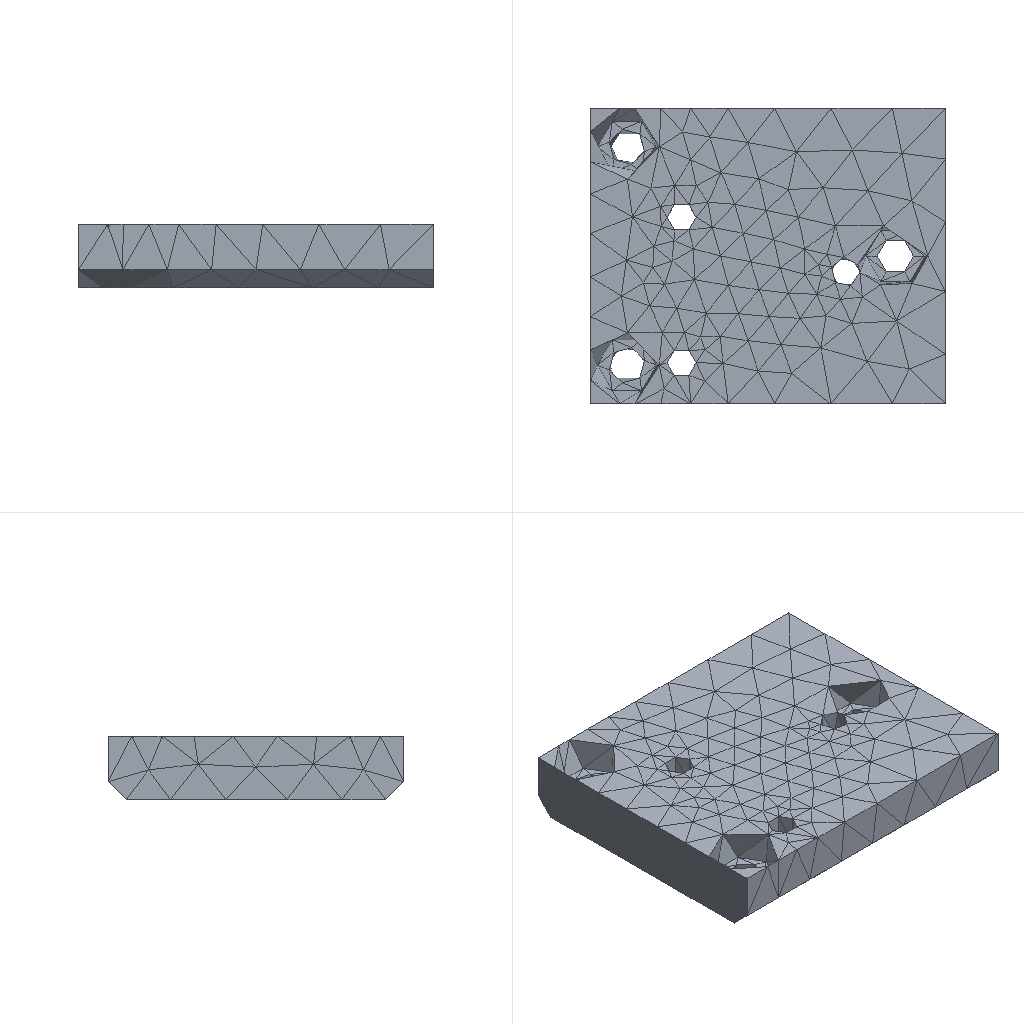Simulation study | nx simcenter
Set-up summary:
category,name,step,type,value,unit,region
solver,nx_nastran (Simcenter)
units,not stated in the deck,,not stated
analysis,deck,,static,static
analysis,solution,,SOL,101
load_step,SUBCASE 1,1,SUBCASE,SPC=1 LOAD=2
load_step,requested,,,1
mesh,nodes,,,2321
mesh,elements,,,1159
element_type,CTETRA,,solid,1159
load,nodal force total,,FX,0.0,model units
load,nodal force total,,FY,0.0,model units
load,nodal force total,,FZ,5000000.063,model units
load,load commands in deck,,count,388
bc,support commands in deck,,count,462
analysis,NX solution 0,,Structural,Linear Statics - Single Constraint
check,setup vs results,,match,every grid point's frame and coordinates and every element id; grid points of CTETRA elements
Nastran input file, long lists of numbers shortened:
$*$$$$$$$$$$$$$$$$$$$$$$$$$$$$$$$$$$$$$$$$$$$$$$$$$$$$$$$$$$$$$$$$$
$*
$*                    NX v10.0.0.24 TRANSLATOR
$*                    FOR NX NASTRAN VERSION 10.0
$ (33 more lines like these left out)
ASSIGN OUTPUT2='116_sim1-solution_1.op2' UNIT=12
$*
$*$$$$$$$$$$$$$$$$$$$$$$$$$$$$$$$$$$$
$*
$* EXECUTIVE CONTROL
$*
$*$$$$$$$$$$$$$$$$$$$$$$$$$$$$$$$$$$$
$*
ID,NASTRAN,116_sim1-solution_1
SOL 101
CEND
$*
$*$$$$$$$$$$$$$$$$$$$$$$$$$$$$$$$$$$$
$*
$* CASE CONTROL
$*
$*$$$$$$$$$$$$$$$$$$$$$$$$$$$$$$$$$$$
$*
TITLE = Solution 1
ECHO = NONE
SPC = 1
OUTPUT
BCRESULTS(TRACTION,FORCE,PLOT) = ALL
DISPLACEMENT(PLOT) = ALL
ESE(PLOT) = ALL
FORCE(PLOT,CORNER) = ALL
OLOAD(PLOT) = ALL
SPCFORCES(PLOT) = ALL
STRAIN(PLOT,FIBER,CORNER) = ALL
STRESS(PLOT,CORNER) = ALL
$*  NX Step: Subcase - Static Loads 1
SUBCASE 1
LABEL = Subcase - Static Loads 1
LOAD = 2
$*
$*$$$$$$$$$$$$$$$$$$$$$$$$$$$$$$$$$$$
$*
$* BULK DATA
$*
$*$$$$$$$$$$$$$$$$$$$$$$$$$$$$$$$$$$$
$*
BEGIN BULK
$*
$* PARAM CARDS
$*
PARAM      K6ROT100.0000
PARAM     OIBULK     YES
PARAM    OMACHPR     YES
PARAM       POST      -2
PARAM    POSTEXT     YES
PARAM    UNITSYS   MN-MM
$*
$* GRID CARDS
$*
GRID*               2281               0-3.310643921E+025.4445001221E+02+
*       3.1089239502E+02               0
GRID*               2282               0-3.310643921E+025.4445001221E+02+
*       3.1589242554E+02               0
$ (4638 more lines like these left out)
$*
$* ELEMENT CARDS
$*
$*  NX Mesh Collector: Solid(1)
$*  NX Mesh: 3d_mesh(1)
CTETRA         1       1       1       2    1572       3      39      40+
+             41      42      43      44
CTETRA         2       1       1    1153       4       5      45      46+
+             47      48      49      50
$ (2314 more lines like these left out)
$*
$* PROPERTY CARDS
$*
$*  NX Property: PSOLID1
PSOLID         1       1       0                           SMECH
$*
$* MATERIAL CARDS
$*
$*  NX Material: Aluminum_6061
MAT1           16.8980+7        0.3300002.7110-62.2161-5
MATT1          1       1               2               3
TABLEM1        1                                                        +
+        20.00006.8980+7 21.11006.8980+7 23.89006.8980+7 37.78006.8290+7+
+        51.67006.8290+7 65.56006.7600+7 79.44006.6910+7 93.33006.6221+7+
+       107.22006.5531+7121.11006.4841+7135.00006.4151+7148.89006.3461+7+
+       162.78006.2772+7176.67006.1392+7190.56006.0702+7204.44005.9323+7+
+       218.33005.8633+7232.22005.7253+7246.11005.5874+7260.00005.4494+7+
+       273.89005.3114+7287.78005.1735+7301.67005.0355+7315.56004.8976+7+
+       329.44004.7596+7343.33004.6216+7357.22004.4147+7371.11004.2767+7+
+       385.00004.1388+7398.89003.9318+7412.78003.7939+7426.67003.5869+7+
+           ENDT
TABLEM1        2                                                        +
+        20.00000.330000 21.11000.330000    ENDT
TABLEM1        3                                                        +
+        20.00002.2380-5 93.33002.3184-5107.22002.3346-5121.11002.3508-5+
+       135.00002.3670-5148.89002.3832-5162.78002.3994-5176.67002.4138-5+
+       190.56002.4300-5204.44002.4444-5218.33002.4588-5232.22002.4732-5+
+       246.11002.4876-5260.00002.5002-5273.89002.5146-5287.78002.5272-5+
+       301.67002.5398-5315.56002.5524-5    ENDT
$*
$* LOAD AND CONSTRAINT CARDS
$*
$*  NX Load and Constraint: Fixed(1)
SPC            1    1567  123456  0.0000
SPC            1    1568  123456  0.0000
SPC            1    1569  123456  0.0000
SPC            1    1570  123456  0.0000
$ (458 more lines like these left out)
$*  NX Load and Constraint: Force(1)
FORCE          2    1235       0 1759.63  0.0000  0.00001.000000
FORCE          2    1236       0 2584.91  0.0000  0.00001.000000
FORCE          2    1237       0 3198.55  0.0000  0.00001.000000
FORCE          2    1238       0 3826.42  0.0000  0.00001.000000
$ (384 more lines like these left out)
ENDDATA dcbedc06
Results summary:
result,analysis,,,static
result,last_loadstep,,,1
result,primary field,,,displacements
result,max displacement,,,0.001106,model units
result,reaction total,,FX,0.02808,model units
result,reaction total,,FY,0.04044,model units
result,reaction total,,FZ,-5000004.0,model units
result,NX solution 0,,loadcases,1,mm